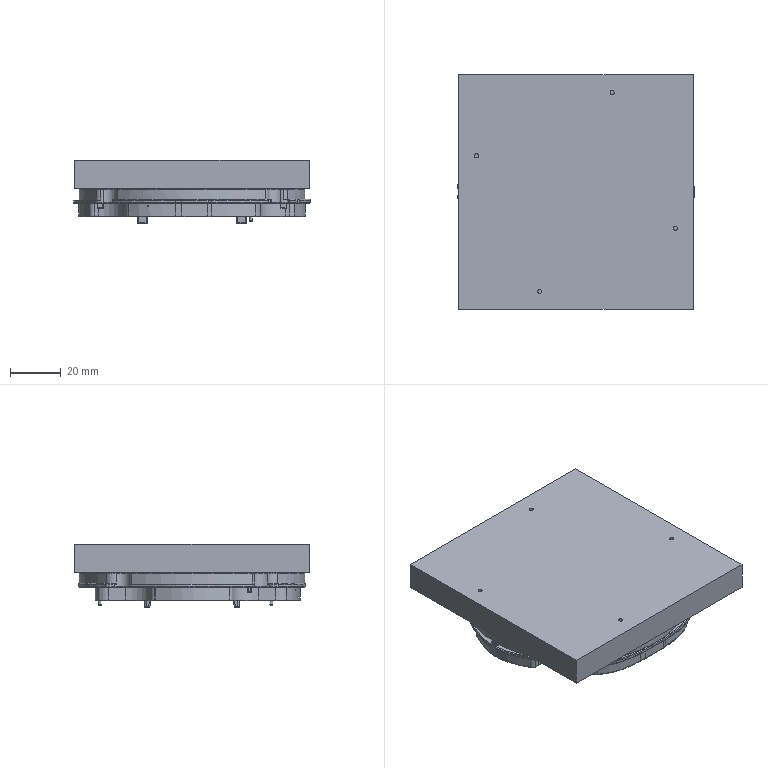NC program | NX | posted with a generic post | part box 92.935 x 92.1 x 24.829 mm
Lines 1 to 863 of 39008:
N10 G17 G21 G94 G90
(PLANAR_MILL_17 , TOOL : D8-25-D8-60-3T-ROUGH)
N12 T10 M6
N14 G54
N16 G17 G0 G90 X21.868 Y34.142 S4500 M3
N18 G43 Z20. H10
N20 Z7.975
N22 G94 G1 X21.849 Y34.119 Z7.974 F1200.
N24 X21.037 Y33.65 Z7.958
N26 X20.112 Y33.496 Z7.941
N28 X19.192 Y33.676 Z7.925
N30 X18.506 Y34.072 Z7.911
N32 X17.872 Y34.81 Z7.894
N34 X17.549 Y35.729 Z7.877
N36 Y36.522 Z7.863
N38 X17.872 Y37.44 Z7.846
N40 X18.506 Y38.179 Z7.829
N42 X19.192 Y38.575 Z7.815
N44 X20.112 Y38.755 Z7.799
N46 X21.037 Y38.601 Z7.783
N48 X21.849 Y38.132 Z7.766
N50 X22.445 Y37.408 Z7.75
N52 X22.749 Y36.522 Z7.734
N54 Y35.729 Z7.72
N56 X22.445 Y34.842 Z7.703
N58 X21.849 Y34.119 Z7.687
N60 X21.037 Y33.65 Z7.671
N62 X20.112 Y33.496 Z7.654
N64 X19.192 Y33.676 Z7.638
N66 X18.506 Y34.072 Z7.624
N68 X17.872 Y34.81 Z7.607
N70 X17.549 Y35.729 Z7.59
N72 Y36.522 Z7.576
N74 X17.872 Y37.44 Z7.559
N76 X18.506 Y38.179 Z7.542
N78 X19.192 Y38.575 Z7.528
N80 X20.112 Y38.755 Z7.512
N82 X21.037 Y38.601 Z7.496
N84 X21.849 Y38.132 Z7.479
N86 X22.445 Y37.408 Z7.463
N88 X22.749 Y36.522 Z7.447
N90 Y35.729 Z7.433
N92 X22.445 Y34.842 Z7.416
N94 X21.849 Y34.119 Z7.4
N96 X21.037 Y33.65 Z7.384
N98 X20.112 Y33.496 Z7.367
N100 X19.192 Y33.676 Z7.351
N102 X18.506 Y34.072 Z7.337
N104 X17.872 Y34.81 Z7.32
N106 X17.549 Y35.729 Z7.303
N108 Y36.522 Z7.289
N110 X17.872 Y37.44 Z7.272
N112 X18.506 Y38.179 Z7.255
N114 X19.192 Y38.575 Z7.242
N116 X20.112 Y38.755 Z7.225
N118 X21.037 Y38.601 Z7.209
N120 X21.849 Y38.132 Z7.192
N122 X22.445 Y37.408 Z7.176
N124 X22.749 Y36.522 Z7.16
N126 Y35.729 Z7.146
N128 X22.445 Y34.842 Z7.13
N130 X21.849 Y34.119 Z7.113
N132 X21.037 Y33.65 Z7.097
N134 X20.112 Y33.496 Z7.08
N136 X19.192 Y33.676 Z7.064
N138 X18.506 Y34.072 Z7.05
N140 X17.872 Y34.81 Z7.033
N142 X17.549 Y35.729 Z7.016
N144 Y36.522 Z7.002
N146 X17.872 Y37.44 Z6.985
N148 X18.506 Y38.179 Z6.968
N150 X19.192 Y38.575 Z6.955
N152 X20.112 Y38.755 Z6.938
N154 X21.037 Y38.601 Z6.922
N156 X21.849 Y38.132 Z6.905
N158 X22.445 Y37.408 Z6.889
N160 X22.749 Y36.522 Z6.873
N162 Y35.729 Z6.859
N164 X22.445 Y34.842 Z6.843
N166 X21.849 Y34.119 Z6.826
N168 X21.037 Y33.65 Z6.81
N170 X20.112 Y33.496 Z6.793
N172 X19.192 Y33.676 Z6.777
N174 X18.506 Y34.072 Z6.763
N176 X17.872 Y34.81 Z6.746
N178 X17.549 Y35.729 Z6.729
N180 Y36.522 Z6.715
N182 X17.872 Y37.44 Z6.698
N184 X18.506 Y38.179 Z6.681
N186 X19.192 Y38.575 Z6.668
N188 X20.112 Y38.755 Z6.651
N190 X21.037 Y38.601 Z6.635
N192 X21.849 Y38.132 Z6.619
N194 X22.445 Y37.408 Z6.602
N196 X22.749 Y36.522 Z6.586
N198 Y35.729 Z6.572
N200 X22.445 Y34.842 Z6.556
N202 X21.849 Y34.119 Z6.539
N204 X21.037 Y33.65 Z6.523
N206 X20.112 Y33.496 Z6.507
N208 X19.192 Y33.676 Z6.49
N210 X18.506 Y34.072 Z6.476
N212 X17.872 Y34.81 Z6.459
N214 X17.549 Y35.729 Z6.442
N216 Y36.522 Z6.428
N218 X17.872 Y37.44 Z6.411
N220 X18.506 Y38.179 Z6.394
N222 X19.192 Y38.575 Z6.381
N224 X20.112 Y38.755 Z6.364
N226 X21.037 Y38.601 Z6.348
N228 X21.849 Y38.132 Z6.332
N230 X22.445 Y37.408 Z6.315
N232 X22.749 Y36.522 Z6.299
N234 Y35.729 Z6.285
N236 X22.445 Y34.842 Z6.269
N238 X21.849 Y34.119 Z6.252
N240 X21.037 Y33.65 Z6.236
N242 X20.112 Y33.496 Z6.22
N244 X19.192 Y33.676 Z6.203
N246 X18.506 Y34.072 Z6.189
N248 X17.872 Y34.81 Z6.172
N250 X17.549 Y35.729 Z6.155
N252 Y36.522 Z6.142
N254 X17.872 Y37.44 Z6.125
N256 X18.506 Y38.179 Z6.108
N258 X19.192 Y38.575 Z6.094
N260 X20.112 Y38.755 Z6.077
N262 X21.037 Y38.601 Z6.061
N264 X21.849 Y38.132 Z6.045
N266 X22.445 Y37.408 Z6.028
N268 X22.749 Y36.522 Z6.012
N270 Y35.729 Z5.998
N272 X22.445 Y34.842 Z5.982
N274 X21.849 Y34.119 Z5.965
N276 X21.037 Y33.65 Z5.949
N278 X20.112 Y33.496 Z5.933
N280 X19.192 Y33.676 Z5.916
N282 X18.506 Y34.072 Z5.902
N284 X17.872 Y34.81 Z5.885
N286 X17.549 Y35.729 Z5.868
N288 Y36.522 Z5.855
N290 X17.872 Y37.44 Z5.838
N292 X18.506 Y38.179 Z5.821
N294 X19.192 Y38.575 Z5.807
N296 X20.112 Y38.755 Z5.79
N298 X21.037 Y38.601 Z5.774
N300 X21.849 Y38.132 Z5.758
N302 X22.445 Y37.408 Z5.741
N304 X22.749 Y36.522 Z5.725
N306 Y35.729 Z5.711
N308 X22.445 Y34.842 Z5.695
N310 X21.849 Y34.119 Z5.678
N312 X21.037 Y33.65 Z5.662
N314 X20.112 Y33.496 Z5.646
N316 X19.192 Y33.676 Z5.629
N318 X18.506 Y34.072 Z5.615
N320 X17.872 Y34.81 Z5.598
N322 X17.549 Y35.729 Z5.581
N324 Y36.522 Z5.568
N326 X17.872 Y37.44 Z5.551
N328 X18.506 Y38.179 Z5.534
N330 X19.192 Y38.575 Z5.52
N332 X20.112 Y38.755 Z5.503
N334 X21.037 Y38.601 Z5.487
N336 X21.849 Y38.132 Z5.471
N338 X22.445 Y37.408 Z5.454
N340 X22.749 Y36.522 Z5.438
N342 Y35.729 Z5.424
N344 X22.445 Y34.842 Z5.408
N346 X21.849 Y34.119 Z5.391
N348 X21.037 Y33.65 Z5.375
N350 X20.112 Y33.496 Z5.359
N352 X19.192 Y33.676 Z5.342
N354 X18.506 Y34.072 Z5.328
N356 X17.872 Y34.81 Z5.311
N358 X17.549 Y35.729 Z5.294
N360 Y36.522 Z5.281
N362 X17.872 Y37.44 Z5.264
N364 X18.506 Y38.179 Z5.247
N366 X19.192 Y38.575 Z5.233
N368 X20.112 Y38.755 Z5.216
N370 X21.037 Y38.601 Z5.2
N372 X21.849 Y38.132 Z5.184
N374 X22.445 Y37.408 Z5.167
N376 X22.749 Y36.522 Z5.151
N378 Y35.729 Z5.137
N380 X22.445 Y34.842 Z5.121
N382 X21.849 Y34.119 Z5.104
N384 X21.037 Y33.65 Z5.088
N386 X20.112 Y33.496 Z5.072
N388 X19.192 Y33.676 Z5.055
N390 X18.506 Y34.072 Z5.042
N392 X17.872 Y34.81 Z5.025
N394 X17.549 Y35.729 Z5.008
N396 Y36.522 Z4.994
N398 X17.872 Y37.44 Z4.977
N400 X18.506 Y38.179 Z4.96
N402 X19.192 Y38.575 Z4.946
N404 X20.112 Y38.755 Z4.93
N406 X21.037 Y38.601 Z4.913
N408 X21.849 Y38.132 Z4.897
N410 X22.445 Y37.408 Z4.88
N412 X22.749 Y36.522 Z4.864
N414 Y35.729 Z4.85
N416 X22.445 Y34.842 Z4.834
N418 X21.849 Y34.119 Z4.817
N420 X21.037 Y33.65 Z4.801
N422 X20.112 Y33.496 Z4.785
N424 X19.192 Y33.676 Z4.768
N426 X18.506 Y34.072 Z4.755
N428 X17.872 Y34.81 Z4.738
N430 X17.549 Y35.729 Z4.721
N432 Y36.522 Z4.707
N434 X17.872 Y37.44 Z4.69
N436 X18.506 Y38.179 Z4.673
N438 X19.192 Y38.575 Z4.659
N440 X20.112 Y38.755 Z4.643
N442 X21.037 Y38.601 Z4.626
N444 X21.849 Y38.132 Z4.61
N446 X22.445 Y37.408 Z4.593
N448 X22.749 Y36.522 Z4.577
N450 Y35.729 Z4.563
N452 X22.445 Y34.842 Z4.547
N454 X21.849 Y34.119 Z4.531
N456 X21.037 Y33.65 Z4.514
N458 X20.112 Y33.496 Z4.498
N460 X19.192 Y33.676 Z4.481
N462 X18.506 Y34.072 Z4.468
N464 X17.872 Y34.81 Z4.451
N466 X17.549 Y35.729 Z4.434
N468 Y36.522 Z4.42
N470 X17.872 Y37.44 Z4.403
N472 X18.506 Y38.179 Z4.386
N474 X19.192 Y38.575 Z4.372
N476 X20.112 Y38.755 Z4.356
N478 X21.037 Y38.601 Z4.339
N480 X21.849 Y38.132 Z4.323
N482 X22.445 Y37.408 Z4.307
N484 X22.749 Y36.522 Z4.29
N486 Y35.729 Z4.276
N488 X22.445 Y34.842 Z4.26
N490 X21.849 Y34.119 Z4.244
N492 X21.037 Y33.65 Z4.227
N494 X20.112 Y33.496 Z4.211
N496 X19.192 Y33.676 Z4.194
N498 X18.506 Y34.072 Z4.181
N500 X17.872 Y34.81 Z4.164
N502 X17.549 Y35.729 Z4.147
N504 Y36.522 Z4.133
N506 X17.872 Y37.44 Z4.116
N508 X18.506 Y38.179 Z4.099
N510 X19.192 Y38.575 Z4.085
N512 X20.112 Y38.755 Z4.069
N514 X21.037 Y38.601 Z4.052
N516 X21.849 Y38.132 Z4.036
N518 X22.445 Y37.408 Z4.02
N520 X22.749 Y36.522 Z4.003
N522 Y35.729 Z3.989
N524 X22.445 Y34.842 Z3.973
N526 X21.849 Y34.119 Z3.957
N528 X21.037 Y33.65 Z3.94
N530 X20.112 Y33.496 Z3.924
N532 X19.192 Y33.676 Z3.908
N534 X18.506 Y34.072 Z3.894
N536 X17.872 Y34.81 Z3.877
N538 X17.549 Y35.729 Z3.86
N540 Y36.522 Z3.846
N542 X17.872 Y37.44 Z3.829
N544 X18.506 Y38.179 Z3.812
N546 X19.192 Y38.575 Z3.798
N548 X20.112 Y38.755 Z3.782
N550 X21.037 Y38.601 Z3.765
N552 X21.849 Y38.132 Z3.749
N554 X22.445 Y37.408 Z3.733
N556 X22.749 Y36.522 Z3.716
N558 Y35.729 Z3.702
N560 X22.445 Y34.842 Z3.686
N562 X21.849 Y34.119 Z3.67
N564 X21.037 Y33.65 Z3.653
N566 X20.112 Y33.496 Z3.637
N568 X19.192 Y33.676 Z3.621
N570 X18.506 Y34.072 Z3.607
N572 X17.872 Y34.81 Z3.59
N574 X17.549 Y35.729 Z3.573
N576 Y36.522 Z3.559
N578 X17.872 Y37.44 Z3.542
N580 X18.506 Y38.179 Z3.525
N582 X19.192 Y38.575 Z3.511
N584 X20.112 Y38.755 Z3.495
N586 X21.037 Y38.601 Z3.478
N588 X21.849 Y38.132 Z3.462
N590 X22.445 Y37.408 Z3.446
N592 X22.749 Y36.522 Z3.429
N594 Y35.729 Z3.415
N596 X22.445 Y34.842 Z3.399
N598 X21.849 Y34.119 Z3.383
N600 X21.037 Y33.65 Z3.366
N602 X20.112 Y33.496 Z3.35
N604 X19.192 Y33.676 Z3.334
N606 X18.506 Y34.072 Z3.32
N608 X17.872 Y34.81 Z3.303
N610 X17.549 Y35.729 Z3.286
N612 Y36.522 Z3.272
N614 X17.872 Y37.44 Z3.255
N616 X18.506 Y38.179 Z3.238
N618 X19.192 Y38.575 Z3.224
N620 X20.112 Y38.755 Z3.208
N622 X21.037 Y38.601 Z3.191
N624 X21.849 Y38.132 Z3.175
N626 X22.445 Y37.408 Z3.159
N628 X22.749 Y36.522 Z3.142
N630 Y35.729 Z3.128
N632 X22.445 Y34.842 Z3.112
N634 X21.849 Y34.119 Z3.096
N636 X21.037 Y33.65 Z3.079
N638 X20.112 Y33.496 Z3.063
N640 X19.192 Y33.676 Z3.047
N642 X18.506 Y34.072 Z3.033
N644 X17.872 Y34.81 Z3.016
N646 X17.549 Y35.729 Z2.999
N648 Y36.522 Z2.985
N650 X17.872 Y37.44 Z2.968
N652 X18.506 Y38.179 Z2.951
N654 X19.192 Y38.575 Z2.937
N656 X20.112 Y38.755 Z2.921
N658 X21.037 Y38.601 Z2.904
N660 X21.849 Y38.132 Z2.888
N662 X22.445 Y37.408 Z2.872
N664 X22.749 Y36.522 Z2.855
N666 Y35.729 Z2.842
N668 X22.445 Y34.842 Z2.825
N670 X21.849 Y34.119 Z2.809
N672 X21.037 Y33.65 Z2.792
N674 X20.112 Y33.496 Z2.776
N676 X19.192 Y33.676 Z2.76
N678 X18.506 Y34.072 Z2.746
N680 X17.872 Y34.81 Z2.729
N682 X17.549 Y35.729 Z2.712
N684 Y36.522 Z2.698
N686 X17.872 Y37.44 Z2.681
N688 X18.506 Y38.179 Z2.664
N690 X19.192 Y38.575 Z2.65
N692 X20.112 Y38.755 Z2.634
N694 X21.037 Y38.601 Z2.618
N696 X21.849 Y38.132 Z2.601
N698 X22.445 Y37.408 Z2.585
N700 X22.749 Y36.522 Z2.568
N702 Y35.729 Z2.555
N704 X22.445 Y34.842 Z2.538
N706 X21.849 Y34.119 Z2.522
N708 X21.037 Y33.65 Z2.505
N710 X20.112 Y33.496 Z2.489
N712 X19.192 Y33.676 Z2.473
N714 X18.506 Y34.072 Z2.459
N716 X17.872 Y34.81 Z2.442
N718 X17.549 Y35.729 Z2.425
N720 Y36.522 Z2.411
N722 X17.872 Y37.44 Z2.394
N724 X18.506 Y38.179 Z2.377
N726 X19.192 Y38.575 Z2.363
N728 X20.112 Y38.755 Z2.347
N730 X21.037 Y38.601 Z2.331
N732 X21.849 Y38.132 Z2.314
N734 X22.445 Y37.408 Z2.298
N736 X22.749 Y36.522 Z2.281
N738 Y35.729 Z2.268
N740 X22.445 Y34.842 Z2.251
N742 X21.849 Y34.119 Z2.235
N744 X21.037 Y33.65 Z2.219
N746 X20.112 Y33.496 Z2.202
N748 X19.192 Y33.676 Z2.186
N750 X18.506 Y34.072 Z2.172
N752 X17.872 Y34.81 Z2.155
N754 X17.549 Y35.729 Z2.138
N756 Y36.522 Z2.124
N758 X17.872 Y37.44 Z2.107
N760 X18.506 Y38.179 Z2.09
N762 X19.192 Y38.575 Z2.076
N764 X20.112 Y38.755 Z2.06
N766 X21.037 Y38.601 Z2.044
N768 X21.849 Y38.132 Z2.027
N770 X22.445 Y37.408 Z2.011
N772 X22.749 Y36.522 Z1.994
N774 Y35.729 Z1.981
N776 X22.445 Y34.842 Z1.964
N778 X21.849 Y34.119 Z1.948
N780 X21.037 Y33.65 Z1.932
N782 X20.112 Y33.496 Z1.915
N784 X19.192 Y33.676 Z1.899
N786 X18.506 Y34.072 Z1.885
N788 X17.872 Y34.81 Z1.868
N790 X17.549 Y35.729 Z1.851
N792 Y36.522 Z1.837
N794 X17.872 Y37.44 Z1.82
N796 X18.506 Y38.179 Z1.803
N798 X19.192 Y38.575 Z1.789
N800 X20.112 Y38.755 Z1.773
N802 X21.037 Y38.601 Z1.757
N804 X21.849 Y38.132 Z1.74
N806 X22.445 Y37.408 Z1.724
N808 X22.749 Y36.522 Z1.708
N810 Y35.729 Z1.694
N812 X22.445 Y34.842 Z1.677
N814 X21.849 Y34.119 Z1.661
N816 X21.037 Y33.65 Z1.645
N818 X20.112 Y33.496 Z1.628
N820 X19.192 Y33.676 Z1.612
N822 X18.506 Y34.072 Z1.598
N824 X17.872 Y34.81 Z1.581
N826 X17.549 Y35.729 Z1.564
N828 Y36.522 Z1.55
N830 X17.872 Y37.44 Z1.533
N832 X18.506 Y38.179 Z1.516
N834 X19.192 Y38.575 Z1.502
N836 X20.112 Y38.755 Z1.486
N838 X21.037 Y38.601 Z1.47
N840 X21.849 Y38.132 Z1.453
N842 X22.445 Y37.408 Z1.437
N844 X22.749 Y36.522 Z1.421
N846 Y35.729 Z1.407
N848 X22.445 Y34.842 Z1.39
N850 X21.849 Y34.119 Z1.374
N852 X21.037 Y33.65 Z1.358
N854 X20.112 Y33.496 Z1.341
N856 X19.192 Y33.676 Z1.325
N858 X18.506 Y34.072 Z1.311
N860 X17.872 Y34.81 Z1.294
N862 X17.549 Y35.729 Z1.277
N864 Y36.522 Z1.263
N866 X17.872 Y37.44 Z1.246
N868 X18.506 Y38.179 Z1.229
N870 X19.192 Y38.575 Z1.215
N872 X20.112 Y38.755 Z1.199
N874 X21.037 Y38.601 Z1.183
N876 X21.849 Y38.132 Z1.166
N878 X22.445 Y37.408 Z1.15
N880 X22.749 Y36.522 Z1.134
N882 Y35.729 Z1.12
N884 X22.445 Y34.842 Z1.103
N886 X21.849 Y34.119 Z1.087
N888 X21.037 Y33.65 Z1.071
N890 X20.112 Y33.496 Z1.054
N892 X19.192 Y33.676 Z1.038
N894 X18.506 Y34.072 Z1.024
N896 X17.872 Y34.81 Z1.007
N898 X17.549 Y35.729 Z0.99
N900 Y36.522 Z0.976
N902 X17.872 Y37.44 Z0.959
N904 X18.506 Y38.179 Z0.942
N906 X19.192 Y38.575 Z0.928
N908 X20.112 Y38.755 Z0.912
N910 X21.037 Y38.601 Z0.896
N912 X21.849 Y38.132 Z0.879
N914 X22.445 Y37.408 Z0.863
N916 X22.749 Y36.522 Z0.847
N918 Y35.729 Z0.833
N920 X22.445 Y34.842 Z0.816
N922 X21.849 Y34.119 Z0.8
N924 X21.037 Y33.65 Z0.784
N926 X20.112 Y33.496 Z0.767
N928 X19.192 Y33.676 Z0.751
N930 X18.506 Y34.072 Z0.737
N932 X17.872 Y34.81 Z0.72
N934 X17.549 Y35.729 Z0.703
N936 Y36.522 Z0.689
N938 X17.872 Y37.44 Z0.672
N940 X18.506 Y38.179 Z0.655
N942 X19.192 Y38.575 Z0.642
N944 X20.112 Y38.755 Z0.625
N946 X21.037 Y38.601 Z0.609
N948 X21.849 Y38.132 Z0.592
N950 X22.445 Y37.408 Z0.576
N952 X22.749 Y36.522 Z0.56
N954 Y35.729 Z0.546
N956 X22.445 Y34.842 Z0.53
N958 X21.849 Y34.119 Z0.513
N960 X21.037 Y33.65 Z0.497
N962 X20.112 Y33.496 Z0.48
N964 X19.192 Y33.676 Z0.464
N966 X18.506 Y34.072 Z0.45
N968 X17.872 Y34.81 Z0.433
N970 X17.549 Y35.729 Z0.416
N972 Y36.522 Z0.402
N974 X17.872 Y37.44 Z0.385
N976 X18.506 Y38.179 Z0.368
N978 X19.192 Y38.575 Z0.355
N980 X20.112 Y38.755 Z0.338
N982 X21.037 Y38.601 Z0.322
N984 X21.849 Y38.132 Z0.305
N986 X22.445 Y37.408 Z0.289
N988 X22.749 Y36.522 Z0.273
N990 Y35.729 Z0.259
N992 X22.445 Y34.842 Z0.243
N994 X21.849 Y34.119 Z0.226
N996 X21.037 Y33.65 Z0.21
N998 X20.112 Y33.496 Z0.193
N1000 X19.192 Y33.676 Z0.177
N1002 X18.506 Y34.072 Z0.163
N1004 X17.872 Y34.81 Z0.146
N1006 X17.549 Y35.729 Z0.129
N1008 Y36.522 Z0.115
N1010 X17.872 Y37.44 Z0.098
N1012 X18.506 Y38.179 Z0.081
N1014 X19.192 Y38.575 Z0.068
N1016 X20.112 Y38.755 Z0.051
N1018 X21.037 Y38.601 Z0.035
N1020 X21.849 Y38.132 Z0.019
N1022 X22.445 Y37.408 Z0.002
N1024 X22.749 Y36.522 Z-0.014
N1026 Y35.729 Z-0.028
N1028 X22.445 Y34.842 Z-0.044
N1030 X21.849 Y34.119 Z-0.061
N1032 X21.037 Y33.65 Z-0.077
N1034 X20.112 Y33.496 Z-0.093
N1036 X19.192 Y33.676 Z-0.11
N1038 X18.506 Y34.072 Z-0.124
N1040 X17.872 Y34.81 Z-0.141
N1042 X17.549 Y35.729 Z-0.158
N1044 Y36.522 Z-0.172
N1046 X17.872 Y37.44 Z-0.189
N1048 X18.506 Y38.179 Z-0.205
N1050 X19.192 Y38.575 Z-0.219
N1052 X20.112 Y38.755 Z-0.236
N1054 X21.037 Y38.601 Z-0.252
N1056 X21.849 Y38.132 Z-0.268
N1058 X22.445 Y37.408 Z-0.285
N1060 X22.749 Y36.522 Z-0.301
N1062 Y35.729 Z-0.315
N1064 X22.445 Y34.842 Z-0.331
N1066 X21.849 Y34.119 Z-0.348
N1068 X21.037 Y33.65 Z-0.364
N1070 X20.112 Y33.496 Z-0.38
N1072 X19.192 Y33.676 Z-0.397
N1074 X18.506 Y34.072 Z-0.411
N1076 X17.872 Y34.81 Z-0.428
N1078 X17.549 Y35.729 Z-0.445
N1080 Y36.522 Z-0.458
N1082 X17.872 Y37.44 Z-0.475
N1084 X18.506 Y38.179 Z-0.492
N1086 X19.192 Y38.575 Z-0.506
N1088 X20.112 Y38.755 Z-0.523
N1090 X21.037 Y38.601 Z-0.539
N1092 X21.849 Y38.132 Z-0.555
N1094 X22.445 Y37.408 Z-0.572
N1096 X22.749 Y36.522 Z-0.588
N1098 Y35.729 Z-0.602
N1100 X22.445 Y34.842 Z-0.618
N1102 X21.849 Y34.119 Z-0.635
N1104 X21.037 Y33.65 Z-0.651
N1106 X20.112 Y33.496 Z-0.667
N1108 X19.192 Y33.676 Z-0.684
N1110 X18.506 Y34.072 Z-0.698
N1112 X17.872 Y34.81 Z-0.715
N1114 X17.549 Y35.729 Z-0.732
N1116 Y36.522 Z-0.745
N1118 X17.872 Y37.44 Z-0.762
N1120 X18.506 Y38.179 Z-0.779
N1122 X19.192 Y38.575 Z-0.793
N1124 X20.112 Y38.755 Z-0.81
N1126 X21.037 Y38.601 Z-0.826
N1128 X21.849 Y38.132 Z-0.842
N1130 X22.445 Y37.408 Z-0.859
N1132 X22.749 Y36.522 Z-0.875
N1134 Y35.729 Z-0.889
N1136 X22.445 Y34.842 Z-0.905
N1138 X21.849 Y34.119 Z-0.922
N1140 X21.037 Y33.65 Z-0.938
N1142 X20.112 Y33.496 Z-0.954
N1144 X19.192 Y33.676 Z-0.971
N1146 X18.506 Y34.072 Z-0.985
N1148 X17.872 Y34.81 Z-1.002
N1150 X17.549 Y35.729 Z-1.019
N1152 Y36.125 Z-1.025
N1154 G2 X20.149 Y38.725 R2.6
N1156 X17.549 Y36.125 R-2.6
N1158 G1 Z0.975
N1160 G0 Z20.
N1162 X-24.865 Y-29.143
N1164 Z7.975
N1166 G1 X-24.846 Y-29.12 Z7.974
N1168 X-24.034 Y-28.651 Z7.958
N1170 X-23.11 Y-28.497 Z7.941
N1172 X-22.189 Y-28.677 Z7.925
N1174 X-21.503 Y-29.073 Z7.911
N1176 X-20.869 Y-29.812 Z7.894
N1178 X-20.546 Y-30.73 Z7.877
N1180 Y-31.523 Z7.863
N1182 X-20.869 Y-32.442 Z7.846
N1184 X-21.503 Y-33.18 Z7.829
N1186 X-22.189 Y-33.576 Z7.815
N1188 X-23.11 Y-33.756 Z7.799
N1190 X-24.034 Y-33.602 Z7.783
N1192 X-24.846 Y-33.133 Z7.766
N1194 X-25.442 Y-32.41 Z7.75
N1196 X-25.746 Y-31.523 Z7.734
N1198 Y-30.73 Z7.72
N1200 X-25.442 Y-29.844 Z7.703
N1202 X-24.846 Y-29.12 Z7.687
N1204 X-24.034 Y-28.651 Z7.671
N1206 X-23.11 Y-28.497 Z7.654
N1208 X-22.189 Y-28.677 Z7.638
N1210 X-21.503 Y-29.073 Z7.624
N1212 X-20.869 Y-29.812 Z7.607
N1214 X-20.546 Y-30.73 Z7.59
N1216 Y-31.523 Z7.576
N1218 X-20.869 Y-32.442 Z7.559
N1220 X-21.503 Y-33.18 Z7.542
N1222 X-22.189 Y-33.576 Z7.528
N1224 X-23.11 Y-33.756 Z7.512
N1226 X-24.034 Y-33.602 Z7.496
N1228 X-24.846 Y-33.133 Z7.479
N1230 X-25.442 Y-32.41 Z7.463
N1232 X-25.746 Y-31.523 Z7.447
N1234 Y-30.73 Z7.433
N1236 X-25.442 Y-29.844 Z7.416
N1238 X-24.846 Y-29.12 Z7.4
N1240 X-24.034 Y-28.651 Z7.384
N1242 X-23.11 Y-28.497 Z7.367
N1244 X-22.189 Y-28.677 Z7.351
N1246 X-21.503 Y-29.073 Z7.337
N1248 X-20.869 Y-29.812 Z7.32
N1250 X-20.546 Y-30.73 Z7.303
N1252 Y-31.523 Z7.289
N1254 X-20.869 Y-32.442 Z7.272
N1256 X-21.503 Y-33.18 Z7.255
N1258 X-22.189 Y-33.576 Z7.242
N1260 X-23.11 Y-33.756 Z7.225
N1262 X-24.034 Y-33.602 Z7.209
N1264 X-24.846 Y-33.133 Z7.192
N1266 X-25.442 Y-32.41 Z7.176
N1268 X-25.746 Y-31.523 Z7.16
N1270 Y-30.73 Z7.146
N1272 X-25.442 Y-29.844 Z7.13
N1274 X-24.846 Y-29.12 Z7.113
N1276 X-24.034 Y-28.651 Z7.097
N1278 X-23.11 Y-28.497 Z7.08
N1280 X-22.189 Y-28.677 Z7.064
N1282 X-21.503 Y-29.073 Z7.05
N1284 X-20.869 Y-29.812 Z7.033
N1286 X-20.546 Y-30.73 Z7.016
N1288 Y-31.523 Z7.002
N1290 X-20.869 Y-32.442 Z6.985
N1292 X-21.503 Y-33.18 Z6.968
N1294 X-22.189 Y-33.576 Z6.955
N1296 X-23.11 Y-33.756 Z6.938
N1298 X-24.034 Y-33.602 Z6.922
N1300 X-24.846 Y-33.133 Z6.905
N1302 X-25.442 Y-32.41 Z6.889
N1304 X-25.746 Y-31.523 Z6.873
N1306 Y-30.73 Z6.859
N1308 X-25.442 Y-29.844 Z6.843
N1310 X-24.846 Y-29.12 Z6.826
N1312 X-24.034 Y-28.651 Z6.81
N1314 X-23.11 Y-28.497 Z6.793
N1316 X-22.189 Y-28.677 Z6.777
N1318 X-21.503 Y-29.073 Z6.763
N1320 X-20.869 Y-29.812 Z6.746
N1322 X-20.546 Y-30.73 Z6.729
N1324 Y-31.523 Z6.715
N1326 X-20.869 Y-32.442 Z6.698
N1328 X-21.503 Y-33.18 Z6.681
N1330 X-22.189 Y-33.576 Z6.668
N1332 X-23.11 Y-33.756 Z6.651
N1334 X-24.034 Y-33.602 Z6.635
N1336 X-24.846 Y-33.133 Z6.619
N1338 X-25.442 Y-32.41 Z6.602
N1340 X-25.746 Y-31.523 Z6.586
N1342 Y-30.73 Z6.572
N1344 X-25.442 Y-29.844 Z6.556
N1346 X-24.846 Y-29.12 Z6.539
N1348 X-24.034 Y-28.651 Z6.523
N1350 X-23.11 Y-28.497 Z6.507
N1352 X-22.189 Y-28.677 Z6.49
N1354 X-21.503 Y-29.073 Z6.476
N1356 X-20.869 Y-29.812 Z6.459
N1358 X-20.546 Y-30.73 Z6.442
N1360 Y-31.523 Z6.428
N1362 X-20.869 Y-32.442 Z6.411
N1364 X-21.503 Y-33.18 Z6.394
N1366 X-22.189 Y-33.576 Z6.381
N1368 X-23.11 Y-33.756 Z6.364
N1370 X-24.034 Y-33.602 Z6.348
N1372 X-24.846 Y-33.133 Z6.332
N1374 X-25.442 Y-32.41 Z6.315
N1376 X-25.746 Y-31.523 Z6.299
N1378 Y-30.73 Z6.285
N1380 X-25.442 Y-29.844 Z6.269
N1382 X-24.846 Y-29.12 Z6.252
N1384 X-24.034 Y-28.651 Z6.236
N1386 X-23.11 Y-28.497 Z6.22
N1388 X-22.189 Y-28.677 Z6.203
N1390 X-21.503 Y-29.073 Z6.189
N1392 X-20.869 Y-29.812 Z6.172
N1394 X-20.546 Y-30.73 Z6.155
N1396 Y-31.523 Z6.142
N1398 X-20.869 Y-32.442 Z6.125
N1400 X-21.503 Y-33.18 Z6.108
N1402 X-22.189 Y-33.576 Z6.094
N1404 X-23.11 Y-33.756 Z6.077
N1406 X-24.034 Y-33.602 Z6.061
N1408 X-24.846 Y-33.133 Z6.045
N1410 X-25.442 Y-32.41 Z6.028
N1412 X-25.746 Y-31.523 Z6.012
N1414 Y-30.73 Z5.998
N1416 X-25.442 Y-29.844 Z5.982
N1418 X-24.846 Y-29.12 Z5.965
N1420 X-24.034 Y-28.651 Z5.949
N1422 X-23.11 Y-28.497 Z5.933
N1424 X-22.189 Y-28.677 Z5.916
N1426 X-21.503 Y-29.073 Z5.902
N1428 X-20.869 Y-29.812 Z5.885
N1430 X-20.546 Y-30.73 Z5.868
N1432 Y-31.523 Z5.855
N1434 X-20.869 Y-32.442 Z5.838
N1436 X-21.503 Y-33.18 Z5.821
N1438 X-22.189 Y-33.576 Z5.807
N1440 X-23.11 Y-33.756 Z5.79
N1442 X-24.034 Y-33.602 Z5.774
N1444 X-24.846 Y-33.133 Z5.758
N1446 X-25.442 Y-32.41 Z5.741
N1448 X-25.746 Y-31.523 Z5.725
N1450 Y-30.73 Z5.711
N1452 X-25.442 Y-29.844 Z5.695
N1454 X-24.846 Y-29.12 Z5.678
N1456 X-24.034 Y-28.651 Z5.662
N1458 X-23.11 Y-28.497 Z5.646
N1460 X-22.189 Y-28.677 Z5.629
N1462 X-21.503 Y-29.073 Z5.615
N1464 X-20.869 Y-29.812 Z5.598
N1466 X-20.546 Y-30.73 Z5.581
N1468 Y-31.523 Z5.568
N1470 X-20.869 Y-32.442 Z5.551
N1472 X-21.503 Y-33.18 Z5.534
N1474 X-22.189 Y-33.576 Z5.52
N1476 X-23.11 Y-33.756 Z5.503
N1478 X-24.034 Y-33.602 Z5.487
N1480 X-24.846 Y-33.133 Z5.471
N1482 X-25.442 Y-32.41 Z5.454
N1484 X-25.746 Y-31.523 Z5.438
N1486 Y-30.73 Z5.424
N1488 X-25.442 Y-29.844 Z5.408
N1490 X-24.846 Y-29.12 Z5.391
N1492 X-24.034 Y-28.651 Z5.375
N1494 X-23.11 Y-28.497 Z5.359
N1496 X-22.189 Y-28.677 Z5.342
N1498 X-21.503 Y-29.073 Z5.328
N1500 X-20.869 Y-29.812 Z5.311
N1502 X-20.546 Y-30.73 Z5.294
N1504 Y-31.523 Z5.281
N1506 X-20.869 Y-32.442 Z5.264
N1508 X-21.503 Y-33.18 Z5.247
N1510 X-22.189 Y-33.576 Z5.233
N1512 X-23.11 Y-33.756 Z5.216
N1514 X-24.034 Y-33.602 Z5.2
N1516 X-24.846 Y-33.133 Z5.184
N1518 X-25.442 Y-32.41 Z5.167
N1520 X-25.746 Y-31.523 Z5.151
N1522 Y-30.73 Z5.137
N1524 X-25.442 Y-29.844 Z5.121
N1526 X-24.846 Y-29.12 Z5.104
N1528 X-24.034 Y-28.651 Z5.088
N1530 X-23.11 Y-28.497 Z5.072
N1532 X-22.189 Y-28.677 Z5.055
N1534 X-21.503 Y-29.073 Z5.042
N1536 X-20.869 Y-29.812 Z5.025
N1538 X-20.546 Y-30.73 Z5.008
N1540 Y-31.523 Z4.994
N1542 X-20.869 Y-32.442 Z4.977
N1544 X-21.503 Y-33.18 Z4.96
N1546 X-22.189 Y-33.576 Z4.946
N1548 X-23.11 Y-33.756 Z4.93
N1550 X-24.034 Y-33.602 Z4.913
N1552 X-24.846 Y-33.133 Z4.897
N1554 X-25.442 Y-32.41 Z4.88
N1556 X-25.746 Y-31.523 Z4.864
N1558 Y-30.73 Z4.85
N1560 X-25.442 Y-29.844 Z4.834
N1562 X-24.846 Y-29.12 Z4.817
N1564 X-24.034 Y-28.651 Z4.801
N1566 X-23.11 Y-28.497 Z4.785
N1568 X-22.189 Y-28.677 Z4.768
N1570 X-21.503 Y-29.073 Z4.755
N1572 X-20.869 Y-29.812 Z4.738
N1574 X-20.546 Y-30.73 Z4.721
N1576 Y-31.523 Z4.707
N1578 X-20.869 Y-32.442 Z4.69
N1580 X-21.503 Y-33.18 Z4.673
N1582 X-22.189 Y-33.576 Z4.659
N1584 X-23.11 Y-33.756 Z4.643
N1586 X-24.034 Y-33.602 Z4.626
N1588 X-24.846 Y-33.133 Z4.61
N1590 X-25.442 Y-32.41 Z4.593
N1592 X-25.746 Y-31.523 Z4.577
N1594 Y-30.73 Z4.563
N1596 X-25.442 Y-29.844 Z4.547
N1598 X-24.846 Y-29.12 Z4.531
N1600 X-24.034 Y-28.651 Z4.514
N1602 X-23.11 Y-28.497 Z4.498
N1604 X-22.189 Y-28.677 Z4.481
N1606 X-21.503 Y-29.073 Z4.468
N1608 X-20.869 Y-29.812 Z4.451
N1610 X-20.546 Y-30.73 Z4.434
N1612 Y-31.523 Z4.42
N1614 X-20.869 Y-32.442 Z4.403
N1616 X-21.503 Y-33.18 Z4.386
N1618 X-22.189 Y-33.576 Z4.372
N1620 X-23.11 Y-33.756 Z4.356
N1622 X-24.034 Y-33.602 Z4.339
N1624 X-24.846 Y-33.133 Z4.323
N1626 X-25.442 Y-32.41 Z4.307
N1628 X-25.746 Y-31.523 Z4.29
N1630 Y-30.73 Z4.276
N1632 X-25.442 Y-29.844 Z4.26
N1634 X-24.846 Y-29.12 Z4.244
N1636 X-24.034 Y-28.651 Z4.227
N1638 X-23.11 Y-28.497 Z4.211
N1640 X-22.189 Y-28.677 Z4.194
N1642 X-21.503 Y-29.073 Z4.181
N1644 X-20.869 Y-29.812 Z4.164
N1646 X-20.546 Y-30.73 Z4.147
N1648 Y-31.523 Z4.133
N1650 X-20.869 Y-32.442 Z4.116
N1652 X-21.503 Y-33.18 Z4.099
N1654 X-22.189 Y-33.576 Z4.085
N1656 X-23.11 Y-33.756 Z4.069
N1658 X-24.034 Y-33.602 Z4.052
N1660 X-24.846 Y-33.133 Z4.036
N1662 X-25.442 Y-32.41 Z4.02
N1664 X-25.746 Y-31.523 Z4.003
N1666 Y-30.73 Z3.989
N1668 X-25.442 Y-29.844 Z3.973
N1670 X-24.846 Y-29.12 Z3.957
N1672 X-24.034 Y-28.651 Z3.94
N1674 X-23.11 Y-28.497 Z3.924
N1676 X-22.189 Y-28.677 Z3.908
N1678 X-21.503 Y-29.073 Z3.894
N1680 X-20.869 Y-29.812 Z3.877
N1682 X-20.546 Y-30.73 Z3.86
N1684 Y-31.523 Z3.846
N1686 X-20.869 Y-32.442 Z3.829
N1688 X-21.503 Y-33.18 Z3.812
N1690 X-22.189 Y-33.576 Z3.798
N1692 X-23.11 Y-33.756 Z3.782
N1694 X-24.034 Y-33.602 Z3.765
N1696 X-24.846 Y-33.133 Z3.749
N1698 X-25.442 Y-32.41 Z3.733
N1700 X-25.746 Y-31.523 Z3.716
N1702 Y-30.73 Z3.702
N1704 X-25.442 Y-29.844 Z3.686
N1706 X-24.846 Y-29.12 Z3.67
N1708 X-24.034 Y-28.651 Z3.653
N1710 X-23.11 Y-28.497 Z3.637
N1712 X-22.189 Y-28.677 Z3.621
N1714 X-21.503 Y-29.073 Z3.607
N1716 X-20.869 Y-29.812 Z3.59
N1718 X-20.546 Y-30.73 Z3.573
N1720 Y-31.523 Z3.559
N1722 X-20.869 Y-32.442 Z3.542
N1724 X-21.503 Y-33.18 Z3.525